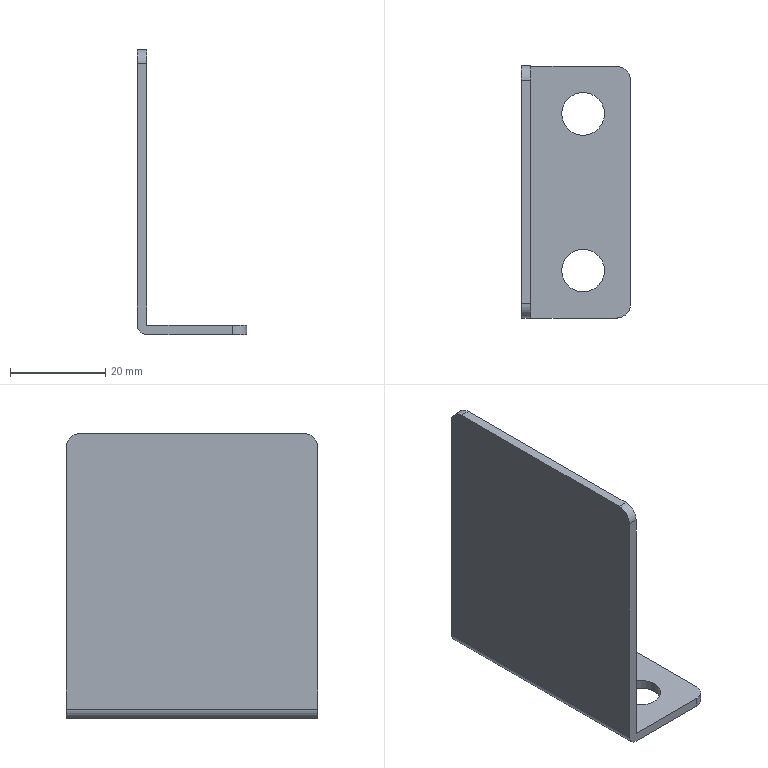Part | STEP file | gslz 2016.10.28-6_id950_x_t | 1 solid | 15 faces | box 23 x 53 x 60 mm | volume 8271 mm3 | plane 8 | cylinder 7 | commonest cylinder face diameters 6 x4 9 x2 4 x1
STEP:
#1=CARTESIAN_POINT('',(101.5,255.5,0.));
#2=VERTEX_POINT('',#1);
#3=CARTESIAN_POINT('',(106.,255.5,0.));
#4=DIRECTION('',(0.,0.,-1.));
#5=DIRECTION('',(-1.,0.,0.));
#6=AXIS2_PLACEMENT_3D('',#3,#4,#5);
#7=CIRCLE('',#6,4.5);
#8=EDGE_CURVE('',#2,#2,#7,.T.);
#9=ORIENTED_EDGE('',*,*,#8,.F.);
#10=EDGE_LOOP('',(#9));
#11=FACE_BOUND('',#10,.T.);
#12=CARTESIAN_POINT('',(116.,262.5,0.));
#13=VERTEX_POINT('',#12);
#14=CARTESIAN_POINT('',(116.,215.5,0.));
#15=VERTEX_POINT('',#14);
#16=CARTESIAN_POINT('',(116.,277.,0.));
#17=DIRECTION('',(0.00000015,-1.,0.));
#18=VECTOR('',#17,1.);
#19=LINE('',#16,#18);
#20=EDGE_CURVE('',#13,#15,#19,.T.);
#21=ORIENTED_EDGE('',*,*,#20,.T.);
#22=CARTESIAN_POINT('',(113.,212.5,0.));
#23=VERTEX_POINT('',#22);
#24=CARTESIAN_POINT('',(113.,215.5,0.));
#25=DIRECTION('',(0.,0.,-1.));
#26=DIRECTION('',(0.,-1.,0.));
#27=AXIS2_PLACEMENT_3D('',#24,#25,#26);
#28=CIRCLE('',#27,3.);
#29=EDGE_CURVE('',#15,#23,#28,.T.);
#30=ORIENTED_EDGE('',*,*,#29,.T.);
#31=CARTESIAN_POINT('',(95.,212.5,0.));
#32=VERTEX_POINT('',#31);
#33=CARTESIAN_POINT('',(-89.45,212.5,0.));
#34=DIRECTION('',(1.,0.,0.));
#35=VECTOR('',#34,1.);
#36=LINE('',#33,#35);
#37=EDGE_CURVE('',#32,#23,#36,.T.);
#38=ORIENTED_EDGE('',*,*,#37,.F.);
#39=CARTESIAN_POINT('',(95.,265.5,0.));
#40=VERTEX_POINT('',#39);
#41=CARTESIAN_POINT('',(95.,265.5,0.));
#42=DIRECTION('',(-0.00000015,1.,0.));
#43=VECTOR('',#42,1.);
#44=LINE('',#41,#43);
#45=EDGE_CURVE('',#32,#40,#44,.T.);
#46=ORIENTED_EDGE('',*,*,#45,.T.);
#47=CARTESIAN_POINT('',(113.,265.5,0.));
#48=VERTEX_POINT('',#47);
#49=CARTESIAN_POINT('',(-89.45,265.5,0.));
#50=DIRECTION('',(1.,0.,0.));
#51=VECTOR('',#50,1.);
#52=LINE('',#49,#51);
#53=EDGE_CURVE('',#40,#48,#52,.T.);
#54=ORIENTED_EDGE('',*,*,#53,.T.);
#55=CARTESIAN_POINT('',(113.,262.5,0.));
#56=DIRECTION('',(0.,0.,-1.));
#57=DIRECTION('',(0.,-1.,0.));
#58=AXIS2_PLACEMENT_3D('',#55,#56,#57);
#59=CIRCLE('',#58,3.);
#60=EDGE_CURVE('',#48,#13,#59,.T.);
#61=ORIENTED_EDGE('',*,*,#60,.T.);
#62=EDGE_LOOP('',(#21,#30,#38,#46,#54,#61));
#63=FACE_BOUND('',#62,.T.);
#64=CARTESIAN_POINT('',(101.5,222.5,0.));
#65=VERTEX_POINT('',#64);
#66=CARTESIAN_POINT('',(106.,222.5,0.));
#67=DIRECTION('',(0.,0.,-1.));
#68=DIRECTION('',(-1.,0.,0.));
#69=AXIS2_PLACEMENT_3D('',#66,#67,#68);
#70=CIRCLE('',#69,4.5);
#71=EDGE_CURVE('',#65,#65,#70,.T.);
#72=ORIENTED_EDGE('',*,*,#71,.F.);
#73=EDGE_LOOP('',(#72));
#74=FACE_BOUND('',#73,.T.);
#75=CARTESIAN_POINT('',(10.55,155.,0.));
#76=DIRECTION('',(0.,0.,1.));
#77=DIRECTION('',(1.,0.,0.));
#78=AXIS2_PLACEMENT_3D('',#75,#76,#77);
#79=PLANE('',#78);
#80=ADVANCED_FACE('',(#11,#63,#74),#79,.F.);
#81=CARTESIAN_POINT('',(101.5,255.5,2.));
#82=VERTEX_POINT('',#81);
#83=CARTESIAN_POINT('',(106.,255.5,2.));
#84=DIRECTION('',(0.,0.,-1.));
#85=DIRECTION('',(-1.,0.,0.));
#86=AXIS2_PLACEMENT_3D('',#83,#84,#85);
#87=CIRCLE('',#86,4.5);
#88=EDGE_CURVE('',#82,#82,#87,.T.);
#89=ORIENTED_EDGE('',*,*,#88,.T.);
#90=EDGE_LOOP('',(#89));
#91=FACE_BOUND('',#90,.T.);
#92=CARTESIAN_POINT('',(95.,212.5,2.));
#93=VERTEX_POINT('',#92);
#94=CARTESIAN_POINT('',(113.,212.5,2.));
#95=VERTEX_POINT('',#94);
#96=CARTESIAN_POINT('',(-89.45,212.5,2.));
#97=DIRECTION('',(1.,0.,0.));
#98=VECTOR('',#97,1.);
#99=LINE('',#96,#98);
#100=EDGE_CURVE('',#93,#95,#99,.T.);
#101=ORIENTED_EDGE('',*,*,#100,.T.);
#102=CARTESIAN_POINT('',(116.,215.5,2.));
#103=VERTEX_POINT('',#102);
#104=CARTESIAN_POINT('',(113.,215.5,2.));
#105=DIRECTION('',(0.,0.,1.));
#106=DIRECTION('',(0.,-1.,0.));
#107=AXIS2_PLACEMENT_3D('',#104,#105,#106);
#108=CIRCLE('',#107,3.);
#109=EDGE_CURVE('',#95,#103,#108,.T.);
#110=ORIENTED_EDGE('',*,*,#109,.T.);
#111=CARTESIAN_POINT('',(116.,262.5,2.));
#112=VERTEX_POINT('',#111);
#113=CARTESIAN_POINT('',(116.,277.,2.));
#114=DIRECTION('',(0.00000015,-1.,0.));
#115=VECTOR('',#114,1.);
#116=LINE('',#113,#115);
#117=EDGE_CURVE('',#112,#103,#116,.T.);
#118=ORIENTED_EDGE('',*,*,#117,.F.);
#119=CARTESIAN_POINT('',(113.,265.5,2.));
#120=VERTEX_POINT('',#119);
#121=CARTESIAN_POINT('',(113.,262.5,2.));
#122=DIRECTION('',(0.,0.,1.));
#123=DIRECTION('',(0.,-1.,0.));
#124=AXIS2_PLACEMENT_3D('',#121,#122,#123);
#125=CIRCLE('',#124,3.);
#126=EDGE_CURVE('',#112,#120,#125,.T.);
#127=ORIENTED_EDGE('',*,*,#126,.T.);
#128=CARTESIAN_POINT('',(95.,265.5,2.));
#129=VERTEX_POINT('',#128);
#130=CARTESIAN_POINT('',(-89.45,265.5,2.));
#131=DIRECTION('',(1.,0.,0.));
#132=VECTOR('',#131,1.);
#133=LINE('',#130,#132);
#134=EDGE_CURVE('',#129,#120,#133,.T.);
#135=ORIENTED_EDGE('',*,*,#134,.F.);
#136=CARTESIAN_POINT('',(95.,264.,2.));
#137=DIRECTION('',(-0.00000015,1.,0.));
#138=VECTOR('',#137,1.);
#139=LINE('',#136,#138);
#140=EDGE_CURVE('',#93,#129,#139,.T.);
#141=ORIENTED_EDGE('',*,*,#140,.F.);
#142=EDGE_LOOP('',(#101,#110,#118,#127,#135,#141));
#143=FACE_BOUND('',#142,.T.);
#144=CARTESIAN_POINT('',(101.5,222.5,2.));
#145=VERTEX_POINT('',#144);
#146=CARTESIAN_POINT('',(106.,222.5,2.));
#147=DIRECTION('',(0.,0.,-1.));
#148=DIRECTION('',(-1.,0.,0.));
#149=AXIS2_PLACEMENT_3D('',#146,#147,#148);
#150=CIRCLE('',#149,4.5);
#151=EDGE_CURVE('',#145,#145,#150,.T.);
#152=ORIENTED_EDGE('',*,*,#151,.T.);
#153=EDGE_LOOP('',(#152));
#154=FACE_BOUND('',#153,.T.);
#155=CARTESIAN_POINT('',(93.,277.,2.));
#156=DIRECTION('',(0.,0.,1.));
#157=DIRECTION('',(1.,0.,0.));
#158=AXIS2_PLACEMENT_3D('',#155,#156,#157);
#159=PLANE('',#158);
#160=ADVANCED_FACE('',(#91,#143,#154),#159,.T.);
#161=ORIENTED_EDGE('',*,*,#134,.T.);
#162=CARTESIAN_POINT('',(113.,265.5,0.));
#163=DIRECTION('',(0.,0.,-1.));
#164=VECTOR('',#163,1.);
#165=LINE('',#162,#164);
#166=EDGE_CURVE('',#120,#48,#165,.T.);
#167=ORIENTED_EDGE('',*,*,#166,.T.);
#168=ORIENTED_EDGE('',*,*,#53,.F.);
#169=CARTESIAN_POINT('',(93.,265.5,2.));
#170=VERTEX_POINT('',#169);
#171=CARTESIAN_POINT('',(95.,265.5,2.));
#172=DIRECTION('',(0.,1.,0.));
#173=DIRECTION('',(-1.,0.,0.));
#174=AXIS2_PLACEMENT_3D('',#171,#172,#173);
#175=CIRCLE('',#174,2.);
#176=EDGE_CURVE('',#40,#170,#175,.T.);
#177=ORIENTED_EDGE('',*,*,#176,.T.);
#178=CARTESIAN_POINT('',(93.,265.5,57.));
#179=VERTEX_POINT('',#178);
#180=CARTESIAN_POINT('',(93.,265.5,2.));
#181=DIRECTION('',(0.,0.,1.));
#182=VECTOR('',#181,1.);
#183=LINE('',#180,#182);
#184=EDGE_CURVE('',#170,#179,#183,.T.);
#185=ORIENTED_EDGE('',*,*,#184,.T.);
#186=CARTESIAN_POINT('',(95.,265.5,57.));
#187=VERTEX_POINT('',#186);
#188=CARTESIAN_POINT('',(-89.45,265.5,57.));
#189=DIRECTION('',(1.,0.,0.));
#190=VECTOR('',#189,1.);
#191=LINE('',#188,#190);
#192=EDGE_CURVE('',#179,#187,#191,.T.);
#193=ORIENTED_EDGE('',*,*,#192,.T.);
#194=CARTESIAN_POINT('',(95.,265.5,2.));
#195=DIRECTION('',(0.,0.,1.));
#196=VECTOR('',#195,1.);
#197=LINE('',#194,#196);
#198=EDGE_CURVE('',#129,#187,#197,.T.);
#199=ORIENTED_EDGE('',*,*,#198,.F.);
#200=EDGE_LOOP('',(#161,#167,#168,#177,#185,#193,#199));
#201=FACE_OUTER_BOUND('',#200,.T.);
#202=CARTESIAN_POINT('',(-89.45,265.5,2.));
#203=DIRECTION('',(0.,1.,0.));
#204=DIRECTION('',(0.,0.,1.));
#205=AXIS2_PLACEMENT_3D('',#202,#203,#204);
#206=PLANE('',#205);
#207=ADVANCED_FACE('',(#201),#206,.T.);
#208=ORIENTED_EDGE('',*,*,#37,.T.);
#209=CARTESIAN_POINT('',(113.,212.5,2.));
#210=DIRECTION('',(0.,0.,1.));
#211=VECTOR('',#210,1.);
#212=LINE('',#209,#211);
#213=EDGE_CURVE('',#23,#95,#212,.T.);
#214=ORIENTED_EDGE('',*,*,#213,.T.);
#215=ORIENTED_EDGE('',*,*,#100,.F.);
#216=CARTESIAN_POINT('',(95.,212.5,57.));
#217=VERTEX_POINT('',#216);
#218=CARTESIAN_POINT('',(95.,212.5,2.));
#219=DIRECTION('',(0.,0.,1.));
#220=VECTOR('',#219,1.);
#221=LINE('',#218,#220);
#222=EDGE_CURVE('',#93,#217,#221,.T.);
#223=ORIENTED_EDGE('',*,*,#222,.T.);
#224=CARTESIAN_POINT('',(93.,212.5,57.));
#225=VERTEX_POINT('',#224);
#226=CARTESIAN_POINT('',(-89.45,212.5,57.));
#227=DIRECTION('',(-1.,0.,0.));
#228=VECTOR('',#227,1.);
#229=LINE('',#226,#228);
#230=EDGE_CURVE('',#217,#225,#229,.T.);
#231=ORIENTED_EDGE('',*,*,#230,.T.);
#232=CARTESIAN_POINT('',(93.,212.5,2.));
#233=VERTEX_POINT('',#232);
#234=CARTESIAN_POINT('',(93.,212.5,2.));
#235=DIRECTION('',(0.,0.,1.));
#236=VECTOR('',#235,1.);
#237=LINE('',#234,#236);
#238=EDGE_CURVE('',#233,#225,#237,.T.);
#239=ORIENTED_EDGE('',*,*,#238,.F.);
#240=CARTESIAN_POINT('',(95.,212.5,2.));
#241=DIRECTION('',(0.,-1.,0.));
#242=DIRECTION('',(-1.,0.,0.));
#243=AXIS2_PLACEMENT_3D('',#240,#241,#242);
#244=CIRCLE('',#243,2.);
#245=EDGE_CURVE('',#233,#32,#244,.T.);
#246=ORIENTED_EDGE('',*,*,#245,.T.);
#247=EDGE_LOOP('',(#208,#214,#215,#223,#231,#239,#246));
#248=FACE_OUTER_BOUND('',#247,.T.);
#249=CARTESIAN_POINT('',(-89.45,212.5,2.));
#250=DIRECTION('',(0.,1.,0.));
#251=DIRECTION('',(0.,0.,1.));
#252=AXIS2_PLACEMENT_3D('',#249,#250,#251);
#253=PLANE('',#252);
#254=ADVANCED_FACE('',(#248),#253,.F.);
#255=CARTESIAN_POINT('',(95.,262.5,60.));
#256=VERTEX_POINT('',#255);
#257=CARTESIAN_POINT('',(95.,215.5,60.));
#258=VERTEX_POINT('',#257);
#259=CARTESIAN_POINT('',(95.,199.,60.));
#260=DIRECTION('',(0.00000015,-1.,0.));
#261=VECTOR('',#260,1.);
#262=LINE('',#259,#261);
#263=EDGE_CURVE('',#256,#258,#262,.T.);
#264=ORIENTED_EDGE('',*,*,#263,.F.);
#265=CARTESIAN_POINT('',(93.,262.5,60.));
#266=VERTEX_POINT('',#265);
#267=CARTESIAN_POINT('',(-89.5,262.5,60.));
#268=DIRECTION('',(-1.,0.,0.));
#269=VECTOR('',#268,1.);
#270=LINE('',#267,#269);
#271=EDGE_CURVE('',#256,#266,#270,.T.);
#272=ORIENTED_EDGE('',*,*,#271,.T.);
#273=CARTESIAN_POINT('',(93.,215.5,60.));
#274=VERTEX_POINT('',#273);
#275=CARTESIAN_POINT('',(93.,199.,60.));
#276=DIRECTION('',(0.00000015,-1.,0.));
#277=VECTOR('',#276,1.);
#278=LINE('',#275,#277);
#279=EDGE_CURVE('',#266,#274,#278,.T.);
#280=ORIENTED_EDGE('',*,*,#279,.T.);
#281=CARTESIAN_POINT('',(-89.5,215.5,60.));
#282=DIRECTION('',(1.,0.,0.));
#283=VECTOR('',#282,1.);
#284=LINE('',#281,#283);
#285=EDGE_CURVE('',#274,#258,#284,.T.);
#286=ORIENTED_EDGE('',*,*,#285,.T.);
#287=EDGE_LOOP('',(#264,#272,#280,#286));
#288=FACE_OUTER_BOUND('',#287,.T.);
#289=CARTESIAN_POINT('',(-89.5,199.,60.));
#290=DIRECTION('',(0.,0.,1.));
#291=DIRECTION('',(-1.,0.,0.));
#292=AXIS2_PLACEMENT_3D('',#289,#290,#291);
#293=PLANE('',#292);
#294=ADVANCED_FACE('',(#288),#293,.T.);
#295=ORIENTED_EDGE('',*,*,#198,.T.);
#296=CARTESIAN_POINT('',(95.,262.5,57.));
#297=DIRECTION('',(1.,0.00000015,0.));
#298=DIRECTION('',(0.00000015,-1.,0.));
#299=AXIS2_PLACEMENT_3D('',#296,#297,#298);
#300=CIRCLE('',#299,3.);
#301=EDGE_CURVE('',#187,#256,#300,.T.);
#302=ORIENTED_EDGE('',*,*,#301,.T.);
#303=ORIENTED_EDGE('',*,*,#263,.T.);
#304=CARTESIAN_POINT('',(95.,215.5,57.));
#305=DIRECTION('',(1.,0.00000015,0.));
#306=DIRECTION('',(0.00000015,-1.,0.));
#307=AXIS2_PLACEMENT_3D('',#304,#305,#306);
#308=CIRCLE('',#307,3.);
#309=EDGE_CURVE('',#258,#217,#308,.T.);
#310=ORIENTED_EDGE('',*,*,#309,.T.);
#311=ORIENTED_EDGE('',*,*,#222,.F.);
#312=ORIENTED_EDGE('',*,*,#140,.T.);
#313=EDGE_LOOP('',(#295,#302,#303,#310,#311,#312));
#314=FACE_OUTER_BOUND('',#313,.T.);
#315=CARTESIAN_POINT('',(95.,264.,-8.));
#316=DIRECTION('',(-1.,-0.00000015,0.));
#317=DIRECTION('',(-0.00000015,1.,0.));
#318=AXIS2_PLACEMENT_3D('',#315,#316,#317);
#319=PLANE('',#318);
#320=ADVANCED_FACE('',(#314),#319,.F.);
#321=ORIENTED_EDGE('',*,*,#279,.F.);
#322=CARTESIAN_POINT('',(93.,262.5,57.));
#323=DIRECTION('',(-1.,-0.00000015,0.));
#324=DIRECTION('',(0.00000015,-1.,0.));
#325=AXIS2_PLACEMENT_3D('',#322,#323,#324);
#326=CIRCLE('',#325,3.);
#327=EDGE_CURVE('',#266,#179,#326,.T.);
#328=ORIENTED_EDGE('',*,*,#327,.T.);
#329=ORIENTED_EDGE('',*,*,#184,.F.);
#330=CARTESIAN_POINT('',(93.,212.5,2.));
#331=DIRECTION('',(0.00000015,-1.,0.));
#332=VECTOR('',#331,1.);
#333=LINE('',#330,#332);
#334=EDGE_CURVE('',#170,#233,#333,.T.);
#335=ORIENTED_EDGE('',*,*,#334,.T.);
#336=ORIENTED_EDGE('',*,*,#238,.T.);
#337=CARTESIAN_POINT('',(93.,215.5,57.));
#338=DIRECTION('',(-1.,-0.00000015,0.));
#339=DIRECTION('',(0.00000015,-1.,0.));
#340=AXIS2_PLACEMENT_3D('',#337,#338,#339);
#341=CIRCLE('',#340,3.);
#342=EDGE_CURVE('',#225,#274,#341,.T.);
#343=ORIENTED_EDGE('',*,*,#342,.T.);
#344=EDGE_LOOP('',(#321,#328,#329,#335,#336,#343));
#345=FACE_OUTER_BOUND('',#344,.T.);
#346=CARTESIAN_POINT('',(93.,264.,-8.));
#347=DIRECTION('',(-1.,-0.00000015,0.));
#348=DIRECTION('',(-0.00000015,1.,0.));
#349=AXIS2_PLACEMENT_3D('',#346,#347,#348);
#350=PLANE('',#349);
#351=ADVANCED_FACE('',(#345),#350,.T.);
#352=ORIENTED_EDGE('',*,*,#117,.T.);
#353=CARTESIAN_POINT('',(116.,215.5,0.));
#354=DIRECTION('',(0.,0.,-1.));
#355=VECTOR('',#354,1.);
#356=LINE('',#353,#355);
#357=EDGE_CURVE('',#103,#15,#356,.T.);
#358=ORIENTED_EDGE('',*,*,#357,.T.);
#359=ORIENTED_EDGE('',*,*,#20,.F.);
#360=CARTESIAN_POINT('',(116.,262.5,2.));
#361=DIRECTION('',(0.,0.,1.));
#362=VECTOR('',#361,1.);
#363=LINE('',#360,#362);
#364=EDGE_CURVE('',#13,#112,#363,.T.);
#365=ORIENTED_EDGE('',*,*,#364,.T.);
#366=EDGE_LOOP('',(#352,#358,#359,#365));
#367=FACE_OUTER_BOUND('',#366,.T.);
#368=CARTESIAN_POINT('',(116.,277.,0.));
#369=DIRECTION('',(-1.,-0.00000015,0.));
#370=DIRECTION('',(-0.00000015,1.,0.));
#371=AXIS2_PLACEMENT_3D('',#368,#369,#370);
#372=PLANE('',#371);
#373=ADVANCED_FACE('',(#367),#372,.F.);
#374=ORIENTED_EDGE('',*,*,#176,.F.);
#375=ORIENTED_EDGE('',*,*,#45,.F.);
#376=ORIENTED_EDGE('',*,*,#245,.F.);
#377=ORIENTED_EDGE('',*,*,#334,.F.);
#378=EDGE_LOOP('',(#374,#375,#376,#377));
#379=FACE_OUTER_BOUND('',#378,.T.);
#380=CARTESIAN_POINT('',(95.,264.,2.));
#381=DIRECTION('',(-0.00000015,1.,0.));
#382=DIRECTION('',(-1.,-0.00000015,0.));
#383=AXIS2_PLACEMENT_3D('',#380,#381,#382);
#384=CYLINDRICAL_SURFACE('',#383,2.);
#385=ADVANCED_FACE('',(#379),#384,.T.);
#386=ORIENTED_EDGE('',*,*,#8,.T.);
#387=EDGE_LOOP('',(#386));
#388=FACE_BOUND('',#387,.T.);
#389=ORIENTED_EDGE('',*,*,#88,.F.);
#390=EDGE_LOOP('',(#389));
#391=FACE_BOUND('',#390,.T.);
#392=CARTESIAN_POINT('',(106.,255.5,0.));
#393=DIRECTION('',(0.,0.,-1.));
#394=DIRECTION('',(-1.,0.,0.));
#395=AXIS2_PLACEMENT_3D('',#392,#393,#394);
#396=CYLINDRICAL_SURFACE('',#395,4.5);
#397=ADVANCED_FACE('',(#388,#391),#396,.F.);
#398=ORIENTED_EDGE('',*,*,#71,.T.);
#399=EDGE_LOOP('',(#398));
#400=FACE_BOUND('',#399,.T.);
#401=ORIENTED_EDGE('',*,*,#151,.F.);
#402=EDGE_LOOP('',(#401));
#403=FACE_BOUND('',#402,.T.);
#404=CARTESIAN_POINT('',(106.,222.5,0.));
#405=DIRECTION('',(0.,0.,-1.));
#406=DIRECTION('',(1.,0.,0.));
#407=AXIS2_PLACEMENT_3D('',#404,#405,#406);
#408=CYLINDRICAL_SURFACE('',#407,4.5);
#409=ADVANCED_FACE('',(#400,#403),#408,.F.);
#410=ORIENTED_EDGE('',*,*,#29,.F.);
#411=ORIENTED_EDGE('',*,*,#357,.F.);
#412=ORIENTED_EDGE('',*,*,#109,.F.);
#413=ORIENTED_EDGE('',*,*,#213,.F.);
#414=EDGE_LOOP('',(#410,#411,#412,#413));
#415=FACE_OUTER_BOUND('',#414,.T.);
#416=CARTESIAN_POINT('',(113.,215.5,2.));
#417=DIRECTION('',(0.,0.,1.));
#418=DIRECTION('',(0.,1.,0.));
#419=AXIS2_PLACEMENT_3D('',#416,#417,#418);
#420=CYLINDRICAL_SURFACE('',#419,3.);
#421=ADVANCED_FACE('',(#415),#420,.T.);
#422=ORIENTED_EDGE('',*,*,#60,.F.);
#423=ORIENTED_EDGE('',*,*,#166,.F.);
#424=ORIENTED_EDGE('',*,*,#126,.F.);
#425=ORIENTED_EDGE('',*,*,#364,.F.);
#426=EDGE_LOOP('',(#422,#423,#424,#425));
#427=FACE_OUTER_BOUND('',#426,.T.);
#428=CARTESIAN_POINT('',(113.,262.5,0.));
#429=DIRECTION('',(0.,0.,-1.));
#430=DIRECTION('',(0.,1.,0.));
#431=AXIS2_PLACEMENT_3D('',#428,#429,#430);
#432=CYLINDRICAL_SURFACE('',#431,3.);
#433=ADVANCED_FACE('',(#427),#432,.T.);
#434=ORIENTED_EDGE('',*,*,#327,.F.);
#435=ORIENTED_EDGE('',*,*,#271,.F.);
#436=ORIENTED_EDGE('',*,*,#301,.F.);
#437=ORIENTED_EDGE('',*,*,#192,.F.);
#438=EDGE_LOOP('',(#434,#435,#436,#437));
#439=FACE_OUTER_BOUND('',#438,.T.);
#440=CARTESIAN_POINT('',(-89.45,262.5,57.));
#441=DIRECTION('',(1.,0.,0.));
#442=DIRECTION('',(0.,1.,0.));
#443=AXIS2_PLACEMENT_3D('',#440,#441,#442);
#444=CYLINDRICAL_SURFACE('',#443,3.);
#445=ADVANCED_FACE('',(#439),#444,.T.);
#446=ORIENTED_EDGE('',*,*,#342,.F.);
#447=ORIENTED_EDGE('',*,*,#230,.F.);
#448=ORIENTED_EDGE('',*,*,#309,.F.);
#449=ORIENTED_EDGE('',*,*,#285,.F.);
#450=EDGE_LOOP('',(#446,#447,#448,#449));
#451=FACE_OUTER_BOUND('',#450,.T.);
#452=CARTESIAN_POINT('',(-89.5,215.5,57.));
#453=DIRECTION('',(-1.,0.,0.));
#454=DIRECTION('',(0.,-1.,0.));
#455=AXIS2_PLACEMENT_3D('',#452,#453,#454);
#456=CYLINDRICAL_SURFACE('',#455,3.);
#457=ADVANCED_FACE('',(#451),#456,.T.);
#458=CLOSED_SHELL('',(#80,#160,#207,#254,#294,#320,#351,#373,#385,#397,#409,#421,#433,#445,#457));
#459=MANIFOLD_SOLID_BREP('',#458);
#460=(LENGTH_UNIT()NAMED_UNIT(*)SI_UNIT(.MILLI.,.METRE.));
#461=UNCERTAINTY_MEASURE_WITH_UNIT(LENGTH_MEASURE(0.00002),#460,'','');
#462=(NAMED_UNIT(*)PLANE_ANGLE_UNIT()SI_UNIT($,.RADIAN.));
#463=PLANE_ANGLE_MEASURE_WITH_UNIT(PLANE_ANGLE_MEASURE(0.01745),#462);
#464=DIMENSIONAL_EXPONENTS(0.,0.,0.,0.,0.,0.,0.);
#465=(CONVERSION_BASED_UNIT('DEGREE',#463)NAMED_UNIT(#464)PLANE_ANGLE_UNIT());
#466=(NAMED_UNIT(*)SI_UNIT($,.STERADIAN.)SOLID_ANGLE_UNIT());
#467=(GEOMETRIC_REPRESENTATION_CONTEXT(3)GLOBAL_UNCERTAINTY_ASSIGNED_CONTEXT((#461))GLOBAL_UNIT_ASSIGNED_CONTEXT((#460,#465,#466))REPRESENTATION_CONTEXT('',''));
#468=ADVANCED_BREP_SHAPE_REPRESENTATION('',(#459),#467);